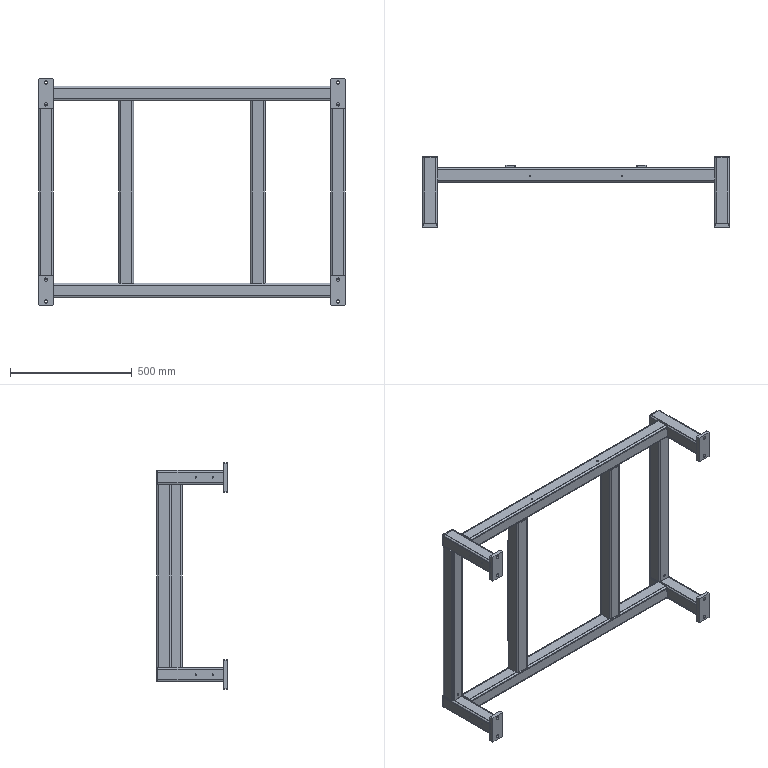Part | SolidWorks | features BaseBody 20 | 20 solids | 366 faces | box 1260 x 290 x 930 mm | volume 5031003 mm3 | plane 190 | cylinder 176 | commonest cylinder face diameters 16 x56 10 x40 5 x24 6.8 x24 9 x16 13.5 x16